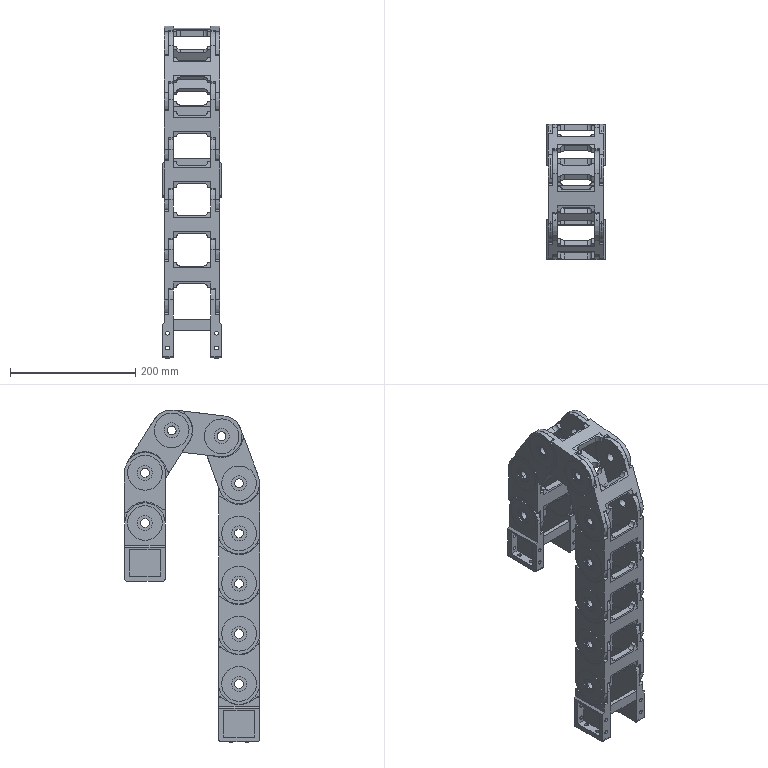Part | SolidWorks | 10 solids | 2438 faces | box 93.598 x 215.392 x 529.568 mm | volume 1411050 mm3 | cylinder 1480 | plane 958 | commonest cylinder face diameters 1 x396 4 x108 2 x96 61.27 x80 24 x72 6 x48